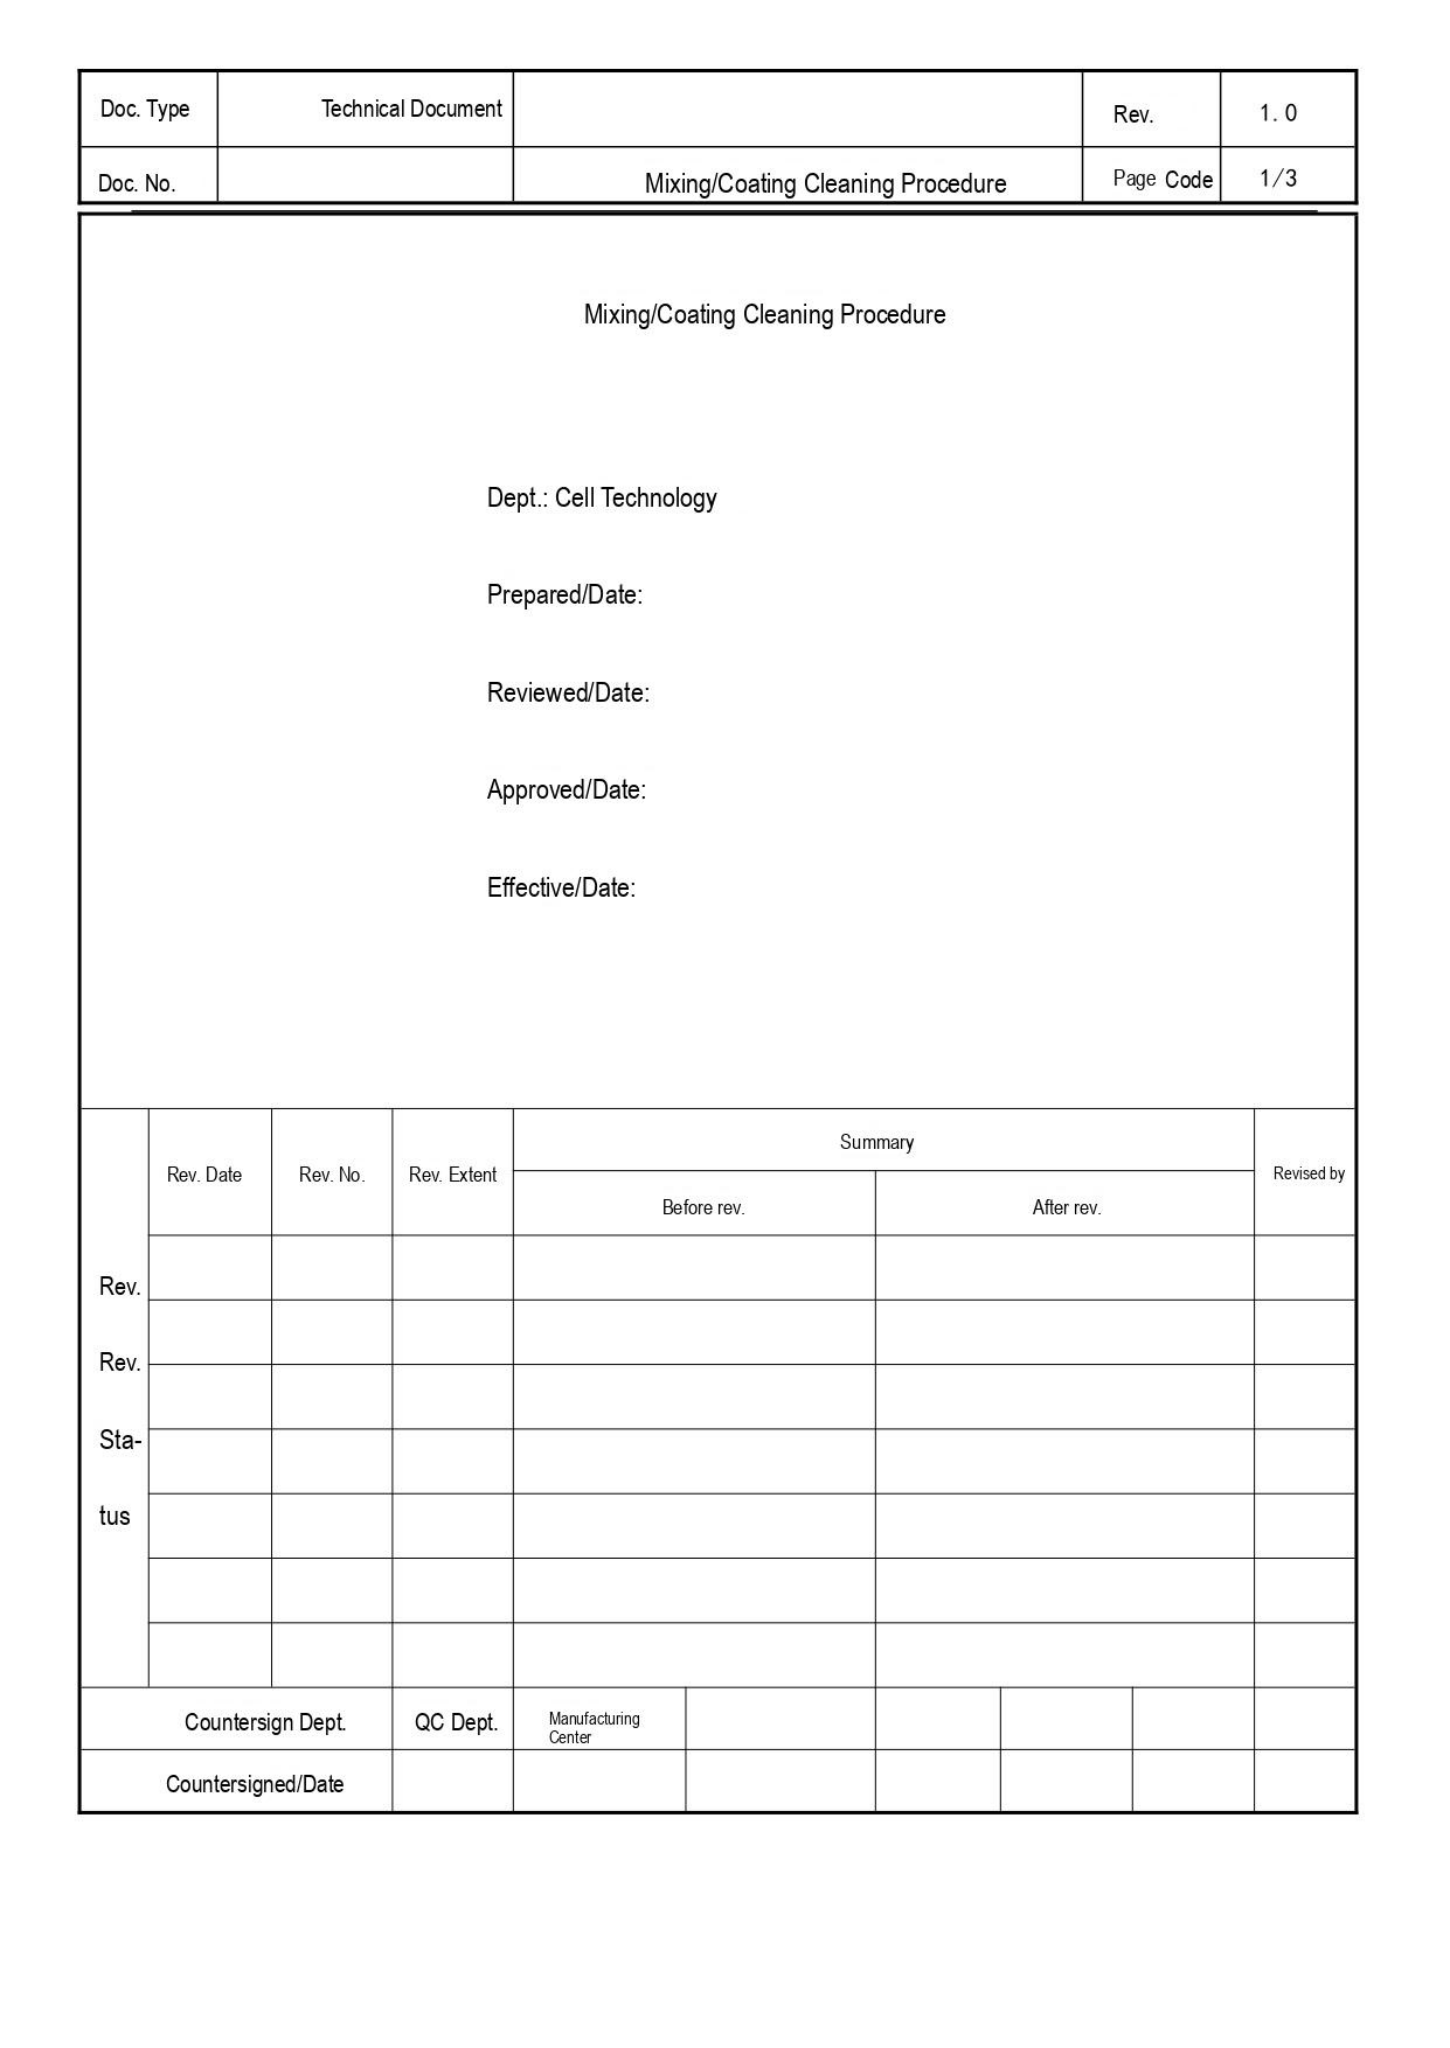| Doc. Type | Technical Document | | Rev. | 1. 0 |
|---|---|---|---|---|
| Doc. No. | | Mixing/Coating Cleaning Procedure | Page Code | 1/3 |

Mixing/Coating Cleaning Procedure

Dept.: Cell Technology

Prepared/Date:

Reviewed/Date:

Approved/Date:

Effective/Date:

| Rev. Rev. Sta-tus | Rev. Date | Rev. No. | Rev. Extent | Summary: Before rev. | Summary: After rev. | Revised by |
|---|---|---|---|---|---|---|
| | | | | | | |
| | | | | | | |
| | | | | | | |
| | | | | | | |
| | | | | | | |
| | | | | | | |
| | | | | | | |

| Countersign Dept. | QC Dept. | Manufacturing Center | | | | | |
|---|---|---|---|---|---|---|---|
| Countersigned/Date | | | | | | | |
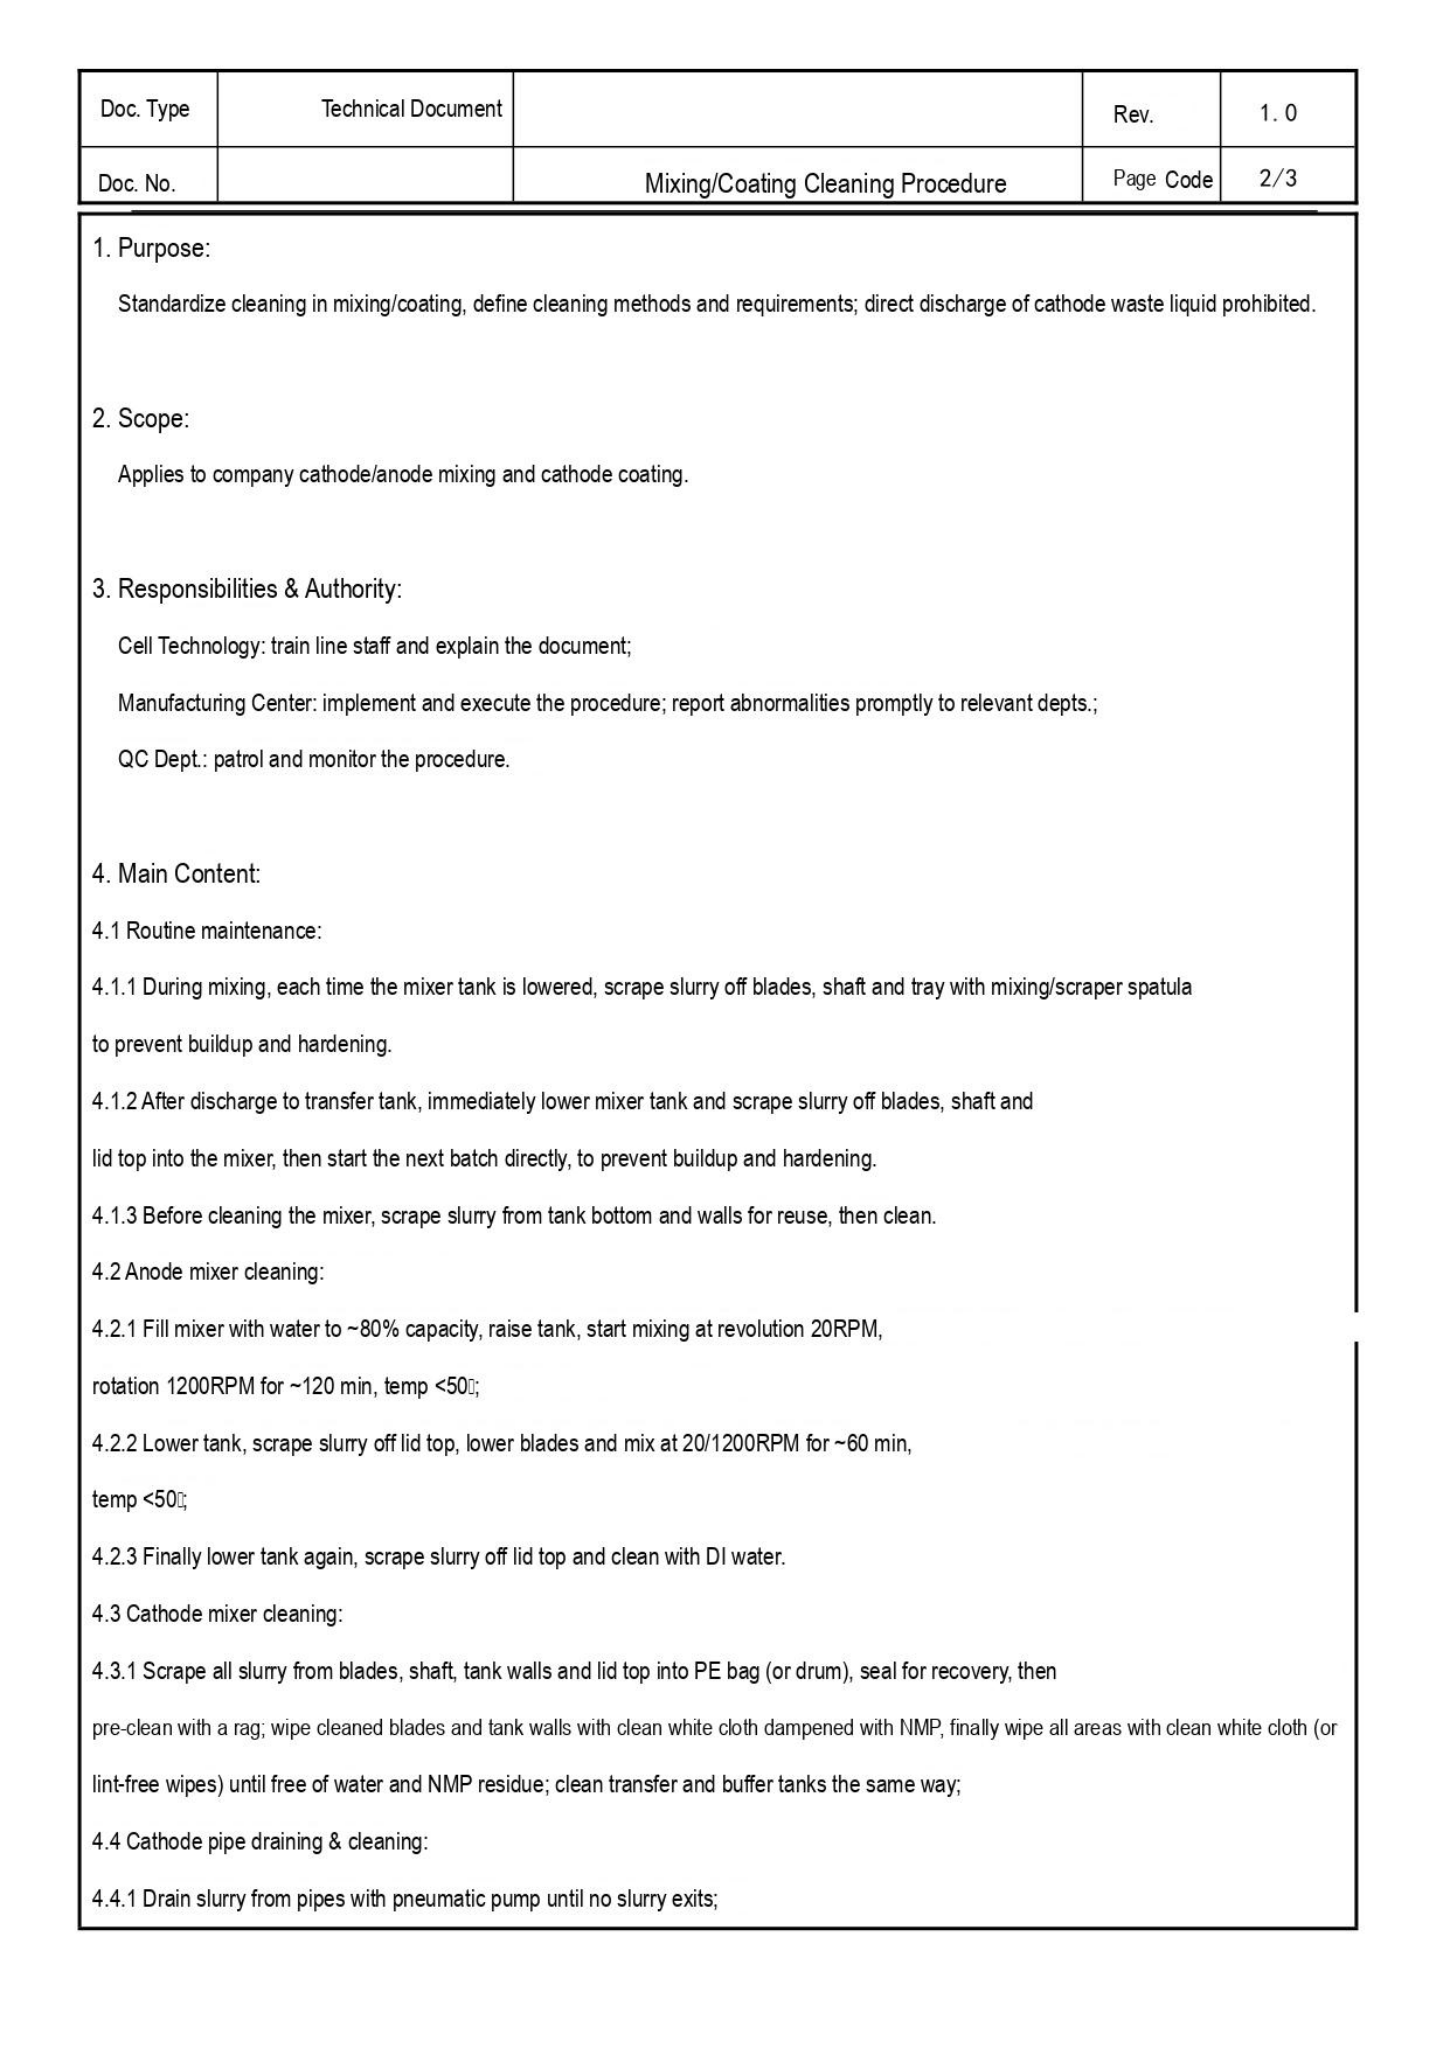| Doc. Type | Technical Document | | Rev. | 1. 0 |
|---|---|---|---|---|
| Doc. No. | | Mixing/Coating Cleaning Procedure | Page Code | 2/3 |

1. Purpose:

Standardize cleaning in mixing/coating, define cleaning methods and requirements; direct discharge of cathode waste liquid prohibited.

2. Scope:

Applies to company cathode/anode mixing and cathode coating.

3. Responsibilities & Authority:

Cell Technology: train line staff and explain the document;

Manufacturing Center: implement and execute the procedure; report abnormalities promptly to relevant depts.;

QC Dept.: patrol and monitor the procedure.

4. Main Content:

4.1 Routine maintenance:

4.1.1 During mixing, each time the mixer tank is lowered, scrape slurry off blades, shaft and tray with mixing/scraper spatula to prevent buildup and hardening.

4.1.2 After discharge to transfer tank, immediately lower mixer tank and scrape slurry off blades, shaft and lid top into the mixer, then start the next batch directly, to prevent buildup and hardening.

4.1.3 Before cleaning the mixer, scrape slurry from tank bottom and walls for reuse, then clean.

4.2 Anode mixer cleaning:

4.2.1 Fill mixer with water to ~80% capacity, raise tank, start mixing at revolution 20RPM, rotation 1200RPM for ~120 min, temp <50;

4.2.2 Lower tank, scrape slurry off lid top, lower blades and mix at 20/1200RPM for ~60 min, temp <50;

4.2.3 Finally lower tank again, scrape slurry off lid top and clean with DI water.

4.3 Cathode mixer cleaning:

4.3.1 Scrape all slurry from blades, shaft, tank walls and lid top into PE bag (or drum), seal for recovery, then pre-clean with a rag; wipe cleaned blades and tank walls with clean white cloth dampened with NMP, finally wipe all areas with clean white cloth (or lint-free wipes) until free of water and NMP residue; clean transfer and buffer tanks the same way;

4.4 Cathode pipe draining & cleaning:

4.4.1 Drain slurry from pipes with pneumatic pump until no slurry exits;
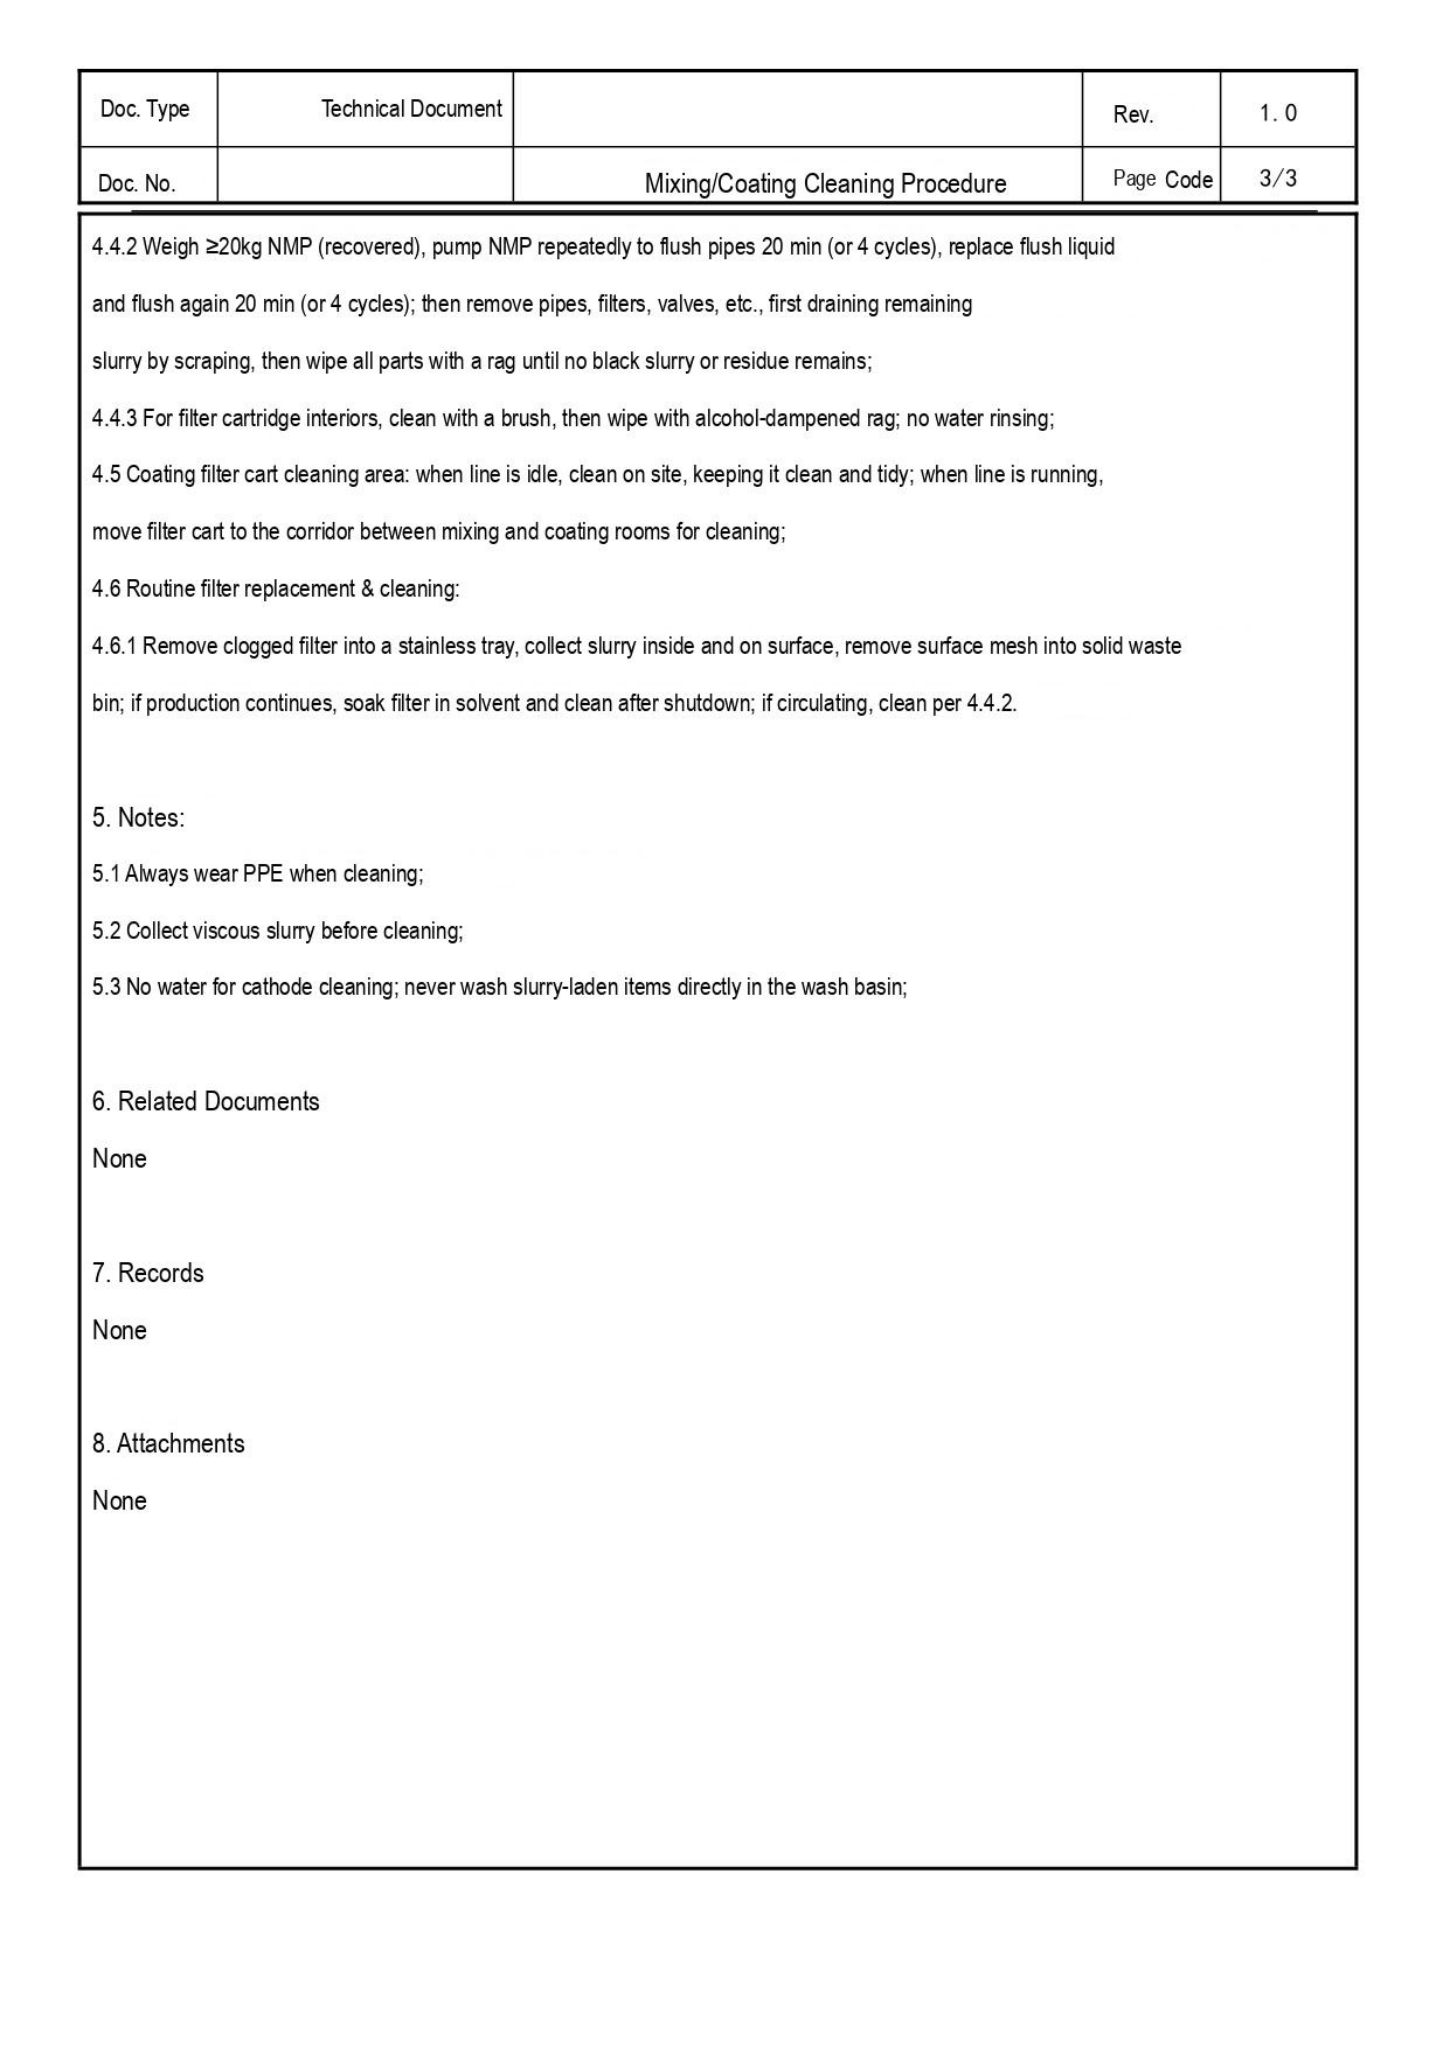| Doc. Type | Technical Document | | Rev. | 1. 0 |
|---|---|---|---|---|
| Doc. No. | | Mixing/Coating Cleaning Procedure | Page Code | 3/3 |

4.4.2 Weigh ≥20kg NMP (recovered), pump NMP repeatedly to flush pipes 20 min (or 4 cycles), replace flush liquid and flush again 20 min (or 4 cycles); then remove pipes, filters, valves, etc., first draining remaining slurry by scraping, then wipe all parts with a rag until no black slurry or residue remains;

4.4.3 For filter cartridge interiors, clean with a brush, then wipe with alcohol-dampened rag; no water rinsing;

4.5 Coating filter cart cleaning area: when line is idle, clean on site, keeping it clean and tidy; when line is running, move filter cart to the corridor between mixing and coating rooms for cleaning;

4.6 Routine filter replacement & cleaning:

4.6.1 Remove clogged filter into a stainless tray, collect slurry inside and on surface, remove surface mesh into solid waste bin; if production continues, soak filter in solvent and clean after shutdown; if circulating, clean per 4.4.2.

5. Notes:

5.1 Always wear PPE when cleaning;

5.2 Collect viscous slurry before cleaning;

5.3 No water for cathode cleaning; never wash slurry-laden items directly in the wash basin;

6. Related Documents

None

7. Records

None

8. Attachments

None